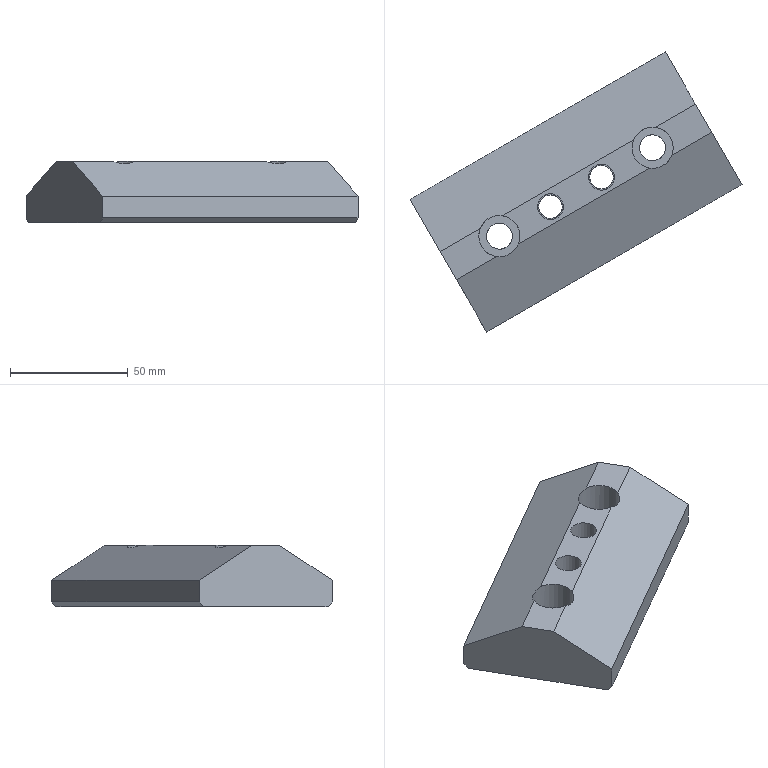Part | NX | features solid 2 | 1 solid | 24 faces | box 140.753 x 118.792 x 26 mm | volume 149536 mm3 | plane 16 | cylinder 8 | commonest cylinder face diameters 11 x4 10 x2 17.5 x2
STEP:
#1=CARTESIAN_POINT('',(-909.878,104.476,-234.));
#2=VERTEX_POINT('',#1);
#3=CARTESIAN_POINT('',(-916.806,116.476,-234.));
#4=VERTEX_POINT('',#3);
#5=CARTESIAN_POINT('',(-917.971,107.804,-234.));
#6=DIRECTION('',(0.,0.,1.));
#7=DIRECTION('',(-0.866,-0.5,0.));
#8=AXIS2_PLACEMENT_3D('',#5,#6,#7);
#9=CIRCLE('',#8,8.75);
#10=EDGE_CURVE('',#2,#4,#9,.T.);
#11=ORIENTED_EDGE('',*,*,#10,.F.);
#12=CARTESIAN_POINT('',(-892.856,114.304,-234.));
#13=VERTEX_POINT('',#12);
#14=CARTESIAN_POINT('',(-892.856,114.304,-234.));
#15=DIRECTION('',(-0.866,-0.5,0.));
#16=VECTOR('',#15,1000.);
#17=LINE('',#14,#16);
#18=EDGE_CURVE('',#13,#2,#17,.T.);
#19=ORIENTED_EDGE('',*,*,#18,.F.);
#20=CARTESIAN_POINT('',(-899.784,126.304,-234.));
#21=VERTEX_POINT('',#20);
#22=CARTESIAN_POINT('',(-899.784,126.304,-234.));
#23=DIRECTION('',(0.5,-0.866,0.));
#24=VECTOR('',#23,1000.);
#25=LINE('',#22,#24);
#26=EDGE_CURVE('',#21,#13,#25,.T.);
#27=ORIENTED_EDGE('',*,*,#26,.F.);
#28=CARTESIAN_POINT('',(-899.784,126.304,-234.));
#29=DIRECTION('',(-0.866,-0.5,0.));
#30=VECTOR('',#29,1000.);
#31=LINE('',#28,#30);
#32=EDGE_CURVE('',#21,#4,#31,.T.);
#33=ORIENTED_EDGE('',*,*,#32,.T.);
#34=EDGE_LOOP('',(#11,#19,#27,#33));
#35=FACE_BOUND('',#34,.T.);
#36=CARTESIAN_POINT('',(-899.784,126.304,-234.));
#37=DIRECTION('',(0.,0.,1.));
#38=DIRECTION('',(-0.5,0.866,0.));
#39=AXIS2_PLACEMENT_3D('',#36,#37,#38);
#40=PLANE('',#39);
#41=ADVANCED_FACE('',(#35),#40,.T.);
#42=CARTESIAN_POINT('',(-944.384,92.554,-234.));
#43=VERTEX_POINT('',#42);
#44=CARTESIAN_POINT('',(-939.621,95.304,-234.));
#45=DIRECTION('',(0.,0.,1.));
#46=DIRECTION('',(-0.866,-0.5,0.));
#47=AXIS2_PLACEMENT_3D('',#44,#45,#46);
#48=CIRCLE('',#47,5.5);
#49=EDGE_CURVE('',#43,#43,#48,.T.);
#50=ORIENTED_EDGE('',*,*,#49,.F.);
#51=EDGE_LOOP('',(#50));
#52=FACE_BOUND('',#51,.T.);
#53=CARTESIAN_POINT('',(-926.063,111.132,-234.));
#54=VERTEX_POINT('',#53);
#55=CARTESIAN_POINT('',(-919.135,99.132,-234.));
#56=VERTEX_POINT('',#55);
#57=CARTESIAN_POINT('',(-917.971,107.804,-234.));
#58=DIRECTION('',(0.,0.,1.));
#59=DIRECTION('',(-0.866,-0.5,0.));
#60=AXIS2_PLACEMENT_3D('',#57,#58,#59);
#61=CIRCLE('',#60,8.75);
#62=EDGE_CURVE('',#54,#56,#61,.T.);
#63=ORIENTED_EDGE('',*,*,#62,.F.);
#64=CARTESIAN_POINT('',(-981.758,78.976,-234.));
#65=VERTEX_POINT('',#64);
#66=CARTESIAN_POINT('',(-899.784,126.304,-234.));
#67=DIRECTION('',(-0.866,-0.5,0.));
#68=VECTOR('',#67,1000.);
#69=LINE('',#66,#68);
#70=EDGE_CURVE('',#54,#65,#69,.T.);
#71=ORIENTED_EDGE('',*,*,#70,.T.);
#72=CARTESIAN_POINT('',(-974.83,66.976,-234.));
#73=VERTEX_POINT('',#72);
#74=CARTESIAN_POINT('',(-982.922,70.304,-234.));
#75=DIRECTION('',(0.,0.,1.));
#76=DIRECTION('',(-0.866,-0.5,0.));
#77=AXIS2_PLACEMENT_3D('',#74,#75,#76);
#78=CIRCLE('',#77,8.75);
#79=EDGE_CURVE('',#73,#65,#78,.T.);
#80=ORIENTED_EDGE('',*,*,#79,.F.);
#81=CARTESIAN_POINT('',(-892.856,114.304,-234.));
#82=DIRECTION('',(-0.866,-0.5,0.));
#83=VECTOR('',#82,1000.);
#84=LINE('',#81,#83);
#85=EDGE_CURVE('',#56,#73,#84,.T.);
#86=ORIENTED_EDGE('',*,*,#85,.F.);
#87=EDGE_LOOP('',(#63,#71,#80,#86));
#88=FACE_BOUND('',#87,.T.);
#89=CARTESIAN_POINT('',(-966.035,80.054,-234.));
#90=VERTEX_POINT('',#89);
#91=CARTESIAN_POINT('',(-961.272,82.804,-234.));
#92=DIRECTION('',(0.,0.,1.));
#93=DIRECTION('',(-0.866,-0.5,0.));
#94=AXIS2_PLACEMENT_3D('',#91,#92,#93);
#95=CIRCLE('',#94,5.5);
#96=EDGE_CURVE('',#90,#90,#95,.T.);
#97=ORIENTED_EDGE('',*,*,#96,.F.);
#98=EDGE_LOOP('',(#97));
#99=FACE_BOUND('',#98,.T.);
#100=CARTESIAN_POINT('',(-899.784,126.304,-234.));
#101=DIRECTION('',(0.,0.,1.));
#102=DIRECTION('',(-0.5,0.866,0.));
#103=AXIS2_PLACEMENT_3D('',#100,#101,#102);
#104=PLANE('',#103);
#105=ADVANCED_FACE('',(#52,#88,#99),#104,.T.);
#106=CARTESIAN_POINT('',(-917.971,107.804,-230.));
#107=DIRECTION('',(-0.25,0.433,-0.866));
#108=DIRECTION('',(0.433,-0.75,-0.5));
#109=AXIS2_PLACEMENT_3D('',#106,#107,#108);
#110=ELLIPSE('',#109,10.104,8.75);
#111=EDGE_CURVE('',#2,#56,#110,.T.);
#112=ORIENTED_EDGE('',*,*,#111,.T.);
#113=ORIENTED_EDGE('',*,*,#85,.T.);
#114=CARTESIAN_POINT('',(-984.087,61.632,-234.));
#115=VERTEX_POINT('',#114);
#116=CARTESIAN_POINT('',(-982.922,70.304,-230.));
#117=DIRECTION('',(-0.25,0.433,-0.866));
#118=DIRECTION('',(0.433,-0.75,-0.5));
#119=AXIS2_PLACEMENT_3D('',#116,#117,#118);
#120=ELLIPSE('',#119,10.104,8.75);
#121=EDGE_CURVE('',#73,#115,#120,.T.);
#122=ORIENTED_EDGE('',*,*,#121,.T.);
#123=CARTESIAN_POINT('',(-1001.109,51.804,-234.));
#124=VERTEX_POINT('',#123);
#125=CARTESIAN_POINT('',(-892.856,114.304,-234.));
#126=DIRECTION('',(-0.866,-0.5,0.));
#127=VECTOR('',#126,1000.);
#128=LINE('',#125,#127);
#129=EDGE_CURVE('',#115,#124,#128,.T.);
#130=ORIENTED_EDGE('',*,*,#129,.T.);
#131=CARTESIAN_POINT('',(-988.323,29.658,-248.764));
#132=VERTEX_POINT('',#131);
#133=CARTESIAN_POINT('',(-1001.109,51.804,-234.));
#134=DIRECTION('',(0.433,-0.75,-0.5));
#135=VECTOR('',#134,1000.);
#136=LINE('',#133,#135);
#137=EDGE_CURVE('',#124,#132,#136,.T.);
#138=ORIENTED_EDGE('',*,*,#137,.T.);
#139=CARTESIAN_POINT('',(-880.07,92.158,-248.764));
#140=VERTEX_POINT('',#139);
#141=CARTESIAN_POINT('',(-880.07,92.158,-248.764));
#142=DIRECTION('',(-0.866,-0.5,0.));
#143=VECTOR('',#142,1000.);
#144=LINE('',#141,#143);
#145=EDGE_CURVE('',#140,#132,#144,.T.);
#146=ORIENTED_EDGE('',*,*,#145,.F.);
#147=CARTESIAN_POINT('',(-892.856,114.304,-234.));
#148=DIRECTION('',(0.433,-0.75,-0.5));
#149=VECTOR('',#148,1000.);
#150=LINE('',#147,#149);
#151=EDGE_CURVE('',#13,#140,#150,.T.);
#152=ORIENTED_EDGE('',*,*,#151,.F.);
#153=ORIENTED_EDGE('',*,*,#18,.T.);
#154=EDGE_LOOP('',(#112,#113,#122,#130,#138,#146,#152,#153));
#155=FACE_BOUND('',#154,.T.);
#156=CARTESIAN_POINT('',(-892.856,114.304,-234.));
#157=DIRECTION('',(0.25,-0.433,0.866));
#158=DIRECTION('',(-0.433,0.75,0.5));
#159=AXIS2_PLACEMENT_3D('',#156,#157,#158);
#160=PLANE('',#159);
#161=ADVANCED_FACE('',(#155),#160,.T.);
#162=CARTESIAN_POINT('',(-880.07,92.158,-258.));
#163=VERTEX_POINT('',#162);
#164=CARTESIAN_POINT('',(-880.07,92.158,-260.));
#165=DIRECTION('',(0.,0.,1.));
#166=VECTOR('',#165,1000.);
#167=LINE('',#164,#166);
#168=EDGE_CURVE('',#163,#140,#167,.T.);
#169=ORIENTED_EDGE('',*,*,#168,.T.);
#170=ORIENTED_EDGE('',*,*,#145,.T.);
#171=CARTESIAN_POINT('',(-988.323,29.658,-258.));
#172=VERTEX_POINT('',#171);
#173=CARTESIAN_POINT('',(-988.323,29.658,-260.));
#174=DIRECTION('',(0.,0.,1.));
#175=VECTOR('',#174,1000.);
#176=LINE('',#173,#175);
#177=EDGE_CURVE('',#172,#132,#176,.T.);
#178=ORIENTED_EDGE('',*,*,#177,.F.);
#179=CARTESIAN_POINT('',(-880.07,92.158,-258.));
#180=DIRECTION('',(-0.866,-0.5,0.));
#181=VECTOR('',#180,1000.);
#182=LINE('',#179,#181);
#183=EDGE_CURVE('',#163,#172,#182,.T.);
#184=ORIENTED_EDGE('',*,*,#183,.F.);
#185=EDGE_LOOP('',(#169,#170,#178,#184));
#186=FACE_BOUND('',#185,.T.);
#187=CARTESIAN_POINT('',(-880.07,92.158,-260.));
#188=DIRECTION('',(-0.5,0.866,0.));
#189=DIRECTION('',(0.,0.,-1.));
#190=AXIS2_PLACEMENT_3D('',#187,#188,#189);
#191=PLANE('',#190);
#192=ADVANCED_FACE('',(#186),#191,.F.);
#193=CARTESIAN_POINT('',(-942.121,99.634,-260.));
#194=VERTEX_POINT('',#193);
#195=CARTESIAN_POINT('',(-939.621,95.304,-260.));
#196=DIRECTION('',(0.,0.,-1.));
#197=DIRECTION('',(-0.5,0.866,0.));
#198=AXIS2_PLACEMENT_3D('',#195,#196,#197);
#199=CIRCLE('',#198,5.);
#200=EDGE_CURVE('',#194,#194,#199,.T.);
#201=ORIENTED_EDGE('',*,*,#200,.F.);
#202=EDGE_LOOP('',(#201));
#203=FACE_BOUND('',#202,.T.);
#204=CARTESIAN_POINT('',(-920.721,112.567,-260.));
#205=VERTEX_POINT('',#204);
#206=CARTESIAN_POINT('',(-917.971,107.804,-260.));
#207=DIRECTION('',(0.,0.,-1.));
#208=DIRECTION('',(-0.5,0.866,0.));
#209=AXIS2_PLACEMENT_3D('',#206,#207,#208);
#210=CIRCLE('',#209,5.5);
#211=EDGE_CURVE('',#205,#205,#210,.T.);
#212=ORIENTED_EDGE('',*,*,#211,.F.);
#213=EDGE_LOOP('',(#212));
#214=FACE_BOUND('',#213,.T.);
#215=CARTESIAN_POINT('',(-963.772,87.134,-260.));
#216=VERTEX_POINT('',#215);
#217=CARTESIAN_POINT('',(-961.272,82.804,-260.));
#218=DIRECTION('',(0.,0.,-1.));
#219=DIRECTION('',(-0.5,0.866,0.));
#220=AXIS2_PLACEMENT_3D('',#217,#218,#219);
#221=CIRCLE('',#220,5.);
#222=EDGE_CURVE('',#216,#216,#221,.T.);
#223=ORIENTED_EDGE('',*,*,#222,.F.);
#224=EDGE_LOOP('',(#223));
#225=FACE_BOUND('',#224,.T.);
#226=CARTESIAN_POINT('',(-985.672,75.067,-260.));
#227=VERTEX_POINT('',#226);
#228=CARTESIAN_POINT('',(-982.922,70.304,-260.));
#229=DIRECTION('',(0.,0.,-1.));
#230=DIRECTION('',(-0.5,0.866,0.));
#231=AXIS2_PLACEMENT_3D('',#228,#229,#230);
#232=CIRCLE('',#231,5.5);
#233=EDGE_CURVE('',#227,#227,#232,.T.);
#234=ORIENTED_EDGE('',*,*,#233,.F.);
#235=EDGE_LOOP('',(#234));
#236=FACE_BOUND('',#235,.T.);
#237=CARTESIAN_POINT('',(-1019.823,84.218,-260.));
#238=VERTEX_POINT('',#237);
#239=CARTESIAN_POINT('',(-989.323,31.391,-260.));
#240=VERTEX_POINT('',#239);
#241=CARTESIAN_POINT('',(-1020.823,85.95,-260.));
#242=DIRECTION('',(0.5,-0.866,0.));
#243=VECTOR('',#242,1000.);
#244=LINE('',#241,#243);
#245=EDGE_CURVE('',#238,#240,#244,.T.);
#246=ORIENTED_EDGE('',*,*,#245,.F.);
#247=CARTESIAN_POINT('',(-911.57,146.718,-260.));
#248=VERTEX_POINT('',#247);
#249=CARTESIAN_POINT('',(-911.57,146.718,-260.));
#250=DIRECTION('',(-0.866,-0.5,0.));
#251=VECTOR('',#250,1000.);
#252=LINE('',#249,#251);
#253=EDGE_CURVE('',#248,#238,#252,.T.);
#254=ORIENTED_EDGE('',*,*,#253,.F.);
#255=CARTESIAN_POINT('',(-881.07,93.891,-260.));
#256=VERTEX_POINT('',#255);
#257=CARTESIAN_POINT('',(-912.57,148.45,-260.));
#258=DIRECTION('',(0.5,-0.866,0.));
#259=VECTOR('',#258,1000.);
#260=LINE('',#257,#259);
#261=EDGE_CURVE('',#248,#256,#260,.T.);
#262=ORIENTED_EDGE('',*,*,#261,.T.);
#263=CARTESIAN_POINT('',(-881.07,93.891,-260.));
#264=DIRECTION('',(0.866,0.5,0.));
#265=VECTOR('',#264,1000.);
#266=LINE('',#263,#265);
#267=EDGE_CURVE('',#240,#256,#266,.T.);
#268=ORIENTED_EDGE('',*,*,#267,.F.);
#269=EDGE_LOOP('',(#246,#254,#262,#268));
#270=FACE_BOUND('',#269,.T.);
#271=CARTESIAN_POINT('',(-912.57,148.45,-260.));
#272=DIRECTION('',(0.,0.,1.));
#273=DIRECTION('',(-0.5,0.866,0.));
#274=AXIS2_PLACEMENT_3D('',#271,#272,#273);
#275=PLANE('',#274);
#276=ADVANCED_FACE('',(#203,#214,#225,#236,#270),#275,.F.);
#277=CARTESIAN_POINT('',(-1020.823,85.95,-248.764));
#278=VERTEX_POINT('',#277);
#279=CARTESIAN_POINT('',(-1020.823,85.95,-258.));
#280=VERTEX_POINT('',#279);
#281=CARTESIAN_POINT('',(-1020.823,85.95,-248.764));
#282=DIRECTION('',(0.,0.,-1.));
#283=VECTOR('',#282,1000.);
#284=LINE('',#281,#283);
#285=EDGE_CURVE('',#278,#280,#284,.T.);
#286=ORIENTED_EDGE('',*,*,#285,.F.);
#287=CARTESIAN_POINT('',(-912.57,148.45,-248.764));
#288=VERTEX_POINT('',#287);
#289=CARTESIAN_POINT('',(-912.57,148.45,-248.764));
#290=DIRECTION('',(-0.866,-0.5,0.));
#291=VECTOR('',#290,1000.);
#292=LINE('',#289,#291);
#293=EDGE_CURVE('',#288,#278,#292,.T.);
#294=ORIENTED_EDGE('',*,*,#293,.F.);
#295=CARTESIAN_POINT('',(-912.57,148.45,-258.));
#296=VERTEX_POINT('',#295);
#297=CARTESIAN_POINT('',(-912.57,148.45,-248.764));
#298=DIRECTION('',(0.,0.,-1.));
#299=VECTOR('',#298,1000.);
#300=LINE('',#297,#299);
#301=EDGE_CURVE('',#288,#296,#300,.T.);
#302=ORIENTED_EDGE('',*,*,#301,.T.);
#303=CARTESIAN_POINT('',(-912.57,148.45,-258.));
#304=DIRECTION('',(0.866,0.5,0.));
#305=VECTOR('',#304,1000.);
#306=LINE('',#303,#305);
#307=EDGE_CURVE('',#280,#296,#306,.T.);
#308=ORIENTED_EDGE('',*,*,#307,.F.);
#309=EDGE_LOOP('',(#286,#294,#302,#308));
#310=FACE_BOUND('',#309,.T.);
#311=CARTESIAN_POINT('',(-912.57,148.45,-248.764));
#312=DIRECTION('',(0.5,-0.866,0.));
#313=DIRECTION('',(0.,0.,1.));
#314=AXIS2_PLACEMENT_3D('',#311,#312,#313);
#315=PLANE('',#314);
#316=ADVANCED_FACE('',(#310),#315,.F.);
#317=CARTESIAN_POINT('',(-917.971,107.804,-230.));
#318=DIRECTION('',(0.25,-0.433,-0.866));
#319=DIRECTION('',(-0.433,0.75,-0.5));
#320=AXIS2_PLACEMENT_3D('',#317,#318,#319);
#321=ELLIPSE('',#320,10.104,8.75);
#322=EDGE_CURVE('',#54,#4,#321,.T.);
#323=ORIENTED_EDGE('',*,*,#322,.T.);
#324=ORIENTED_EDGE('',*,*,#32,.F.);
#325=CARTESIAN_POINT('',(-912.57,148.45,-248.764));
#326=DIRECTION('',(0.433,-0.75,0.5));
#327=VECTOR('',#326,1000.);
#328=LINE('',#325,#327);
#329=EDGE_CURVE('',#288,#21,#328,.T.);
#330=ORIENTED_EDGE('',*,*,#329,.F.);
#331=ORIENTED_EDGE('',*,*,#293,.T.);
#332=CARTESIAN_POINT('',(-1008.037,63.804,-234.));
#333=VERTEX_POINT('',#332);
#334=CARTESIAN_POINT('',(-1020.823,85.95,-248.764));
#335=DIRECTION('',(0.433,-0.75,0.5));
#336=VECTOR('',#335,1000.);
#337=LINE('',#334,#336);
#338=EDGE_CURVE('',#278,#333,#337,.T.);
#339=ORIENTED_EDGE('',*,*,#338,.T.);
#340=CARTESIAN_POINT('',(-991.015,73.632,-234.));
#341=VERTEX_POINT('',#340);
#342=CARTESIAN_POINT('',(-899.784,126.304,-234.));
#343=DIRECTION('',(-0.866,-0.5,0.));
#344=VECTOR('',#343,1000.);
#345=LINE('',#342,#344);
#346=EDGE_CURVE('',#341,#333,#345,.T.);
#347=ORIENTED_EDGE('',*,*,#346,.F.);
#348=CARTESIAN_POINT('',(-982.922,70.304,-230.));
#349=DIRECTION('',(0.25,-0.433,-0.866));
#350=DIRECTION('',(-0.433,0.75,-0.5));
#351=AXIS2_PLACEMENT_3D('',#348,#349,#350);
#352=ELLIPSE('',#351,10.104,8.75);
#353=EDGE_CURVE('',#341,#65,#352,.T.);
#354=ORIENTED_EDGE('',*,*,#353,.T.);
#355=ORIENTED_EDGE('',*,*,#70,.F.);
#356=EDGE_LOOP('',(#323,#324,#330,#331,#339,#347,#354,#355));
#357=FACE_BOUND('',#356,.T.);
#358=CARTESIAN_POINT('',(-912.57,148.45,-248.764));
#359=DIRECTION('',(-0.25,0.433,0.866));
#360=DIRECTION('',(-0.433,0.75,-0.5));
#361=AXIS2_PLACEMENT_3D('',#358,#359,#360);
#362=PLANE('',#361);
#363=ADVANCED_FACE('',(#357),#362,.T.);
#364=CARTESIAN_POINT('',(-982.922,70.304,-234.));
#365=DIRECTION('',(0.,0.,-1.));
#366=DIRECTION('',(-0.5,0.866,0.));
#367=AXIS2_PLACEMENT_3D('',#364,#365,#366);
#368=CIRCLE('',#367,8.75);
#369=EDGE_CURVE('',#115,#341,#368,.T.);
#370=ORIENTED_EDGE('',*,*,#369,.T.);
#371=ORIENTED_EDGE('',*,*,#346,.T.);
#372=CARTESIAN_POINT('',(-1008.037,63.804,-234.));
#373=DIRECTION('',(0.5,-0.866,0.));
#374=VECTOR('',#373,1000.);
#375=LINE('',#372,#374);
#376=EDGE_CURVE('',#333,#124,#375,.T.);
#377=ORIENTED_EDGE('',*,*,#376,.T.);
#378=ORIENTED_EDGE('',*,*,#129,.F.);
#379=EDGE_LOOP('',(#370,#371,#377,#378));
#380=FACE_BOUND('',#379,.T.);
#381=CARTESIAN_POINT('',(-899.784,126.304,-234.));
#382=DIRECTION('',(0.,0.,1.));
#383=DIRECTION('',(-0.5,0.866,0.));
#384=AXIS2_PLACEMENT_3D('',#381,#382,#383);
#385=PLANE('',#384);
#386=ADVANCED_FACE('',(#380),#385,.T.);
#387=ORIENTED_EDGE('',*,*,#261,.F.);
#388=CARTESIAN_POINT('',(-911.445,146.502,-260.25));
#389=DIRECTION('',(-0.3536,0.6124,0.7071));
#390=VECTOR('',#389,1000.);
#391=LINE('',#388,#390);
#392=EDGE_CURVE('',#296,#248,#391,.F.);
#393=ORIENTED_EDGE('',*,*,#392,.F.);
#394=ORIENTED_EDGE('',*,*,#301,.F.);
#395=ORIENTED_EDGE('',*,*,#329,.T.);
#396=ORIENTED_EDGE('',*,*,#26,.T.);
#397=ORIENTED_EDGE('',*,*,#151,.T.);
#398=ORIENTED_EDGE('',*,*,#168,.F.);
#399=CARTESIAN_POINT('',(-881.195,94.107,-260.25));
#400=DIRECTION('',(-0.3536,0.6124,-0.7071));
#401=VECTOR('',#400,1000.);
#402=LINE('',#399,#401);
#403=EDGE_CURVE('',#256,#163,#402,.F.);
#404=ORIENTED_EDGE('',*,*,#403,.F.);
#405=EDGE_LOOP('',(#387,#393,#394,#395,#396,#397,#398,#404));
#406=FACE_BOUND('',#405,.T.);
#407=CARTESIAN_POINT('',(-896.32,120.304,-230.));
#408=DIRECTION('',(0.866,0.5,0.));
#409=DIRECTION('',(0.,0.,-1.));
#410=AXIS2_PLACEMENT_3D('',#407,#408,#409);
#411=PLANE('',#410);
#412=ADVANCED_FACE('',(#406),#411,.T.);
#413=ORIENTED_EDGE('',*,*,#177,.T.);
#414=ORIENTED_EDGE('',*,*,#137,.F.);
#415=ORIENTED_EDGE('',*,*,#376,.F.);
#416=ORIENTED_EDGE('',*,*,#338,.F.);
#417=ORIENTED_EDGE('',*,*,#285,.T.);
#418=CARTESIAN_POINT('',(-1019.823,84.218,-260.));
#419=DIRECTION('',(0.3536,-0.6124,-0.7071));
#420=VECTOR('',#419,1000.);
#421=LINE('',#418,#420);
#422=EDGE_CURVE('',#238,#280,#421,.F.);
#423=ORIENTED_EDGE('',*,*,#422,.F.);
#424=ORIENTED_EDGE('',*,*,#245,.T.);
#425=CARTESIAN_POINT('',(-988.323,29.658,-258.));
#426=DIRECTION('',(0.3536,-0.6124,0.7071));
#427=VECTOR('',#426,1000.);
#428=LINE('',#425,#427);
#429=EDGE_CURVE('',#172,#240,#428,.F.);
#430=ORIENTED_EDGE('',*,*,#429,.F.);
#431=EDGE_LOOP('',(#413,#414,#415,#416,#417,#423,#424,#430));
#432=FACE_BOUND('',#431,.T.);
#433=CARTESIAN_POINT('',(-1004.573,57.804,-230.));
#434=DIRECTION('',(0.866,0.5,0.));
#435=DIRECTION('',(0.,0.,-1.));
#436=AXIS2_PLACEMENT_3D('',#433,#434,#435);
#437=PLANE('',#436);
#438=ADVANCED_FACE('',(#432),#437,.F.);
#439=CARTESIAN_POINT('',(-987.686,67.554,-250.));
#440=VERTEX_POINT('',#439);
#441=CARTESIAN_POINT('',(-982.922,70.304,-250.));
#442=DIRECTION('',(0.,0.,1.));
#443=DIRECTION('',(-0.866,-0.5,0.));
#444=AXIS2_PLACEMENT_3D('',#441,#442,#443);
#445=CIRCLE('',#444,5.5);
#446=EDGE_CURVE('',#440,#440,#445,.T.);
#447=ORIENTED_EDGE('',*,*,#446,.T.);
#448=EDGE_LOOP('',(#447));
#449=FACE_BOUND('',#448,.T.);
#450=ORIENTED_EDGE('',*,*,#233,.T.);
#451=EDGE_LOOP('',(#450));
#452=FACE_BOUND('',#451,.T.);
#453=CARTESIAN_POINT('',(-982.922,70.304,-264.));
#454=DIRECTION('',(0.,0.,-1.));
#455=DIRECTION('',(-0.866,-0.5,0.));
#456=AXIS2_PLACEMENT_3D('',#453,#454,#455);
#457=CYLINDRICAL_SURFACE('',#456,5.5);
#458=ADVANCED_FACE('',(#449,#452),#457,.F.);
#459=ORIENTED_EDGE('',*,*,#446,.F.);
#460=EDGE_LOOP('',(#459));
#461=FACE_BOUND('',#460,.T.);
#462=CARTESIAN_POINT('',(-990.5,65.929,-250.));
#463=VERTEX_POINT('',#462);
#464=CARTESIAN_POINT('',(-982.922,70.304,-250.));
#465=DIRECTION('',(0.,0.,1.));
#466=DIRECTION('',(-0.866,-0.5,0.));
#467=AXIS2_PLACEMENT_3D('',#464,#465,#466);
#468=CIRCLE('',#467,8.75);
#469=EDGE_CURVE('',#463,#463,#468,.T.);
#470=ORIENTED_EDGE('',*,*,#469,.T.);
#471=EDGE_LOOP('',(#470));
#472=FACE_BOUND('',#471,.T.);
#473=CARTESIAN_POINT('',(-982.922,70.304,-250.));
#474=DIRECTION('',(0.,0.,-1.));
#475=DIRECTION('',(-0.866,-0.5,0.));
#476=AXIS2_PLACEMENT_3D('',#473,#474,#475);
#477=PLANE('',#476);
#478=ADVANCED_FACE('',(#461,#472),#477,.F.);
#479=ORIENTED_EDGE('',*,*,#121,.F.);
#480=ORIENTED_EDGE('',*,*,#79,.T.);
#481=ORIENTED_EDGE('',*,*,#353,.F.);
#482=ORIENTED_EDGE('',*,*,#369,.F.);
#483=EDGE_LOOP('',(#479,#480,#481,#482));
#484=FACE_BOUND('',#483,.T.);
#485=ORIENTED_EDGE('',*,*,#469,.F.);
#486=EDGE_LOOP('',(#485));
#487=FACE_BOUND('',#486,.T.);
#488=CARTESIAN_POINT('',(-982.922,70.304,-234.));
#489=DIRECTION('',(0.,0.,-1.));
#490=DIRECTION('',(-0.866,-0.5,0.));
#491=AXIS2_PLACEMENT_3D('',#488,#489,#490);
#492=CYLINDRICAL_SURFACE('',#491,8.75);
#493=ADVANCED_FACE('',(#484,#487),#492,.F.);
#494=CARTESIAN_POINT('',(-965.602,80.304,-245.));
#495=VERTEX_POINT('',#494);
#496=CARTESIAN_POINT('',(-961.272,82.804,-245.));
#497=DIRECTION('',(0.,0.,1.));
#498=DIRECTION('',(-0.866,-0.5,0.));
#499=AXIS2_PLACEMENT_3D('',#496,#497,#498);
#500=CIRCLE('',#499,5.);
#501=EDGE_CURVE('',#495,#495,#500,.T.);
#502=ORIENTED_EDGE('',*,*,#501,.T.);
#503=EDGE_LOOP('',(#502));
#504=FACE_BOUND('',#503,.T.);
#505=ORIENTED_EDGE('',*,*,#222,.T.);
#506=EDGE_LOOP('',(#505));
#507=FACE_BOUND('',#506,.T.);
#508=CARTESIAN_POINT('',(-961.272,82.804,-264.));
#509=DIRECTION('',(0.,0.,-1.));
#510=DIRECTION('',(-0.866,-0.5,0.));
#511=AXIS2_PLACEMENT_3D('',#508,#509,#510);
#512=CYLINDRICAL_SURFACE('',#511,5.);
#513=ADVANCED_FACE('',(#504,#507),#512,.F.);
#514=ORIENTED_EDGE('',*,*,#501,.F.);
#515=EDGE_LOOP('',(#514));
#516=FACE_BOUND('',#515,.T.);
#517=CARTESIAN_POINT('',(-966.035,80.054,-245.));
#518=VERTEX_POINT('',#517);
#519=CARTESIAN_POINT('',(-961.272,82.804,-245.));
#520=DIRECTION('',(0.,0.,1.));
#521=DIRECTION('',(-0.866,-0.5,0.));
#522=AXIS2_PLACEMENT_3D('',#519,#520,#521);
#523=CIRCLE('',#522,5.5);
#524=EDGE_CURVE('',#518,#518,#523,.T.);
#525=ORIENTED_EDGE('',*,*,#524,.T.);
#526=EDGE_LOOP('',(#525));
#527=FACE_BOUND('',#526,.T.);
#528=CARTESIAN_POINT('',(-961.272,82.804,-245.));
#529=DIRECTION('',(0.,0.,-1.));
#530=DIRECTION('',(-0.866,-0.5,0.));
#531=AXIS2_PLACEMENT_3D('',#528,#529,#530);
#532=PLANE('',#531);
#533=ADVANCED_FACE('',(#516,#527),#532,.F.);
#534=ORIENTED_EDGE('',*,*,#524,.F.);
#535=EDGE_LOOP('',(#534));
#536=FACE_BOUND('',#535,.T.);
#537=ORIENTED_EDGE('',*,*,#96,.T.);
#538=EDGE_LOOP('',(#537));
#539=FACE_BOUND('',#538,.T.);
#540=CARTESIAN_POINT('',(-961.272,82.804,-234.));
#541=DIRECTION('',(0.,0.,-1.));
#542=DIRECTION('',(-0.866,-0.5,0.));
#543=AXIS2_PLACEMENT_3D('',#540,#541,#542);
#544=CYLINDRICAL_SURFACE('',#543,5.5);
#545=ADVANCED_FACE('',(#536,#539),#544,.F.);
#546=CARTESIAN_POINT('',(-922.734,105.054,-250.));
#547=VERTEX_POINT('',#546);
#548=CARTESIAN_POINT('',(-917.971,107.804,-250.));
#549=DIRECTION('',(0.,0.,1.));
#550=DIRECTION('',(-0.866,-0.5,0.));
#551=AXIS2_PLACEMENT_3D('',#548,#549,#550);
#552=CIRCLE('',#551,5.5);
#553=EDGE_CURVE('',#547,#547,#552,.T.);
#554=ORIENTED_EDGE('',*,*,#553,.T.);
#555=EDGE_LOOP('',(#554));
#556=FACE_BOUND('',#555,.T.);
#557=ORIENTED_EDGE('',*,*,#211,.T.);
#558=EDGE_LOOP('',(#557));
#559=FACE_BOUND('',#558,.T.);
#560=CARTESIAN_POINT('',(-917.971,107.804,-264.));
#561=DIRECTION('',(0.,0.,-1.));
#562=DIRECTION('',(-0.866,-0.5,0.));
#563=AXIS2_PLACEMENT_3D('',#560,#561,#562);
#564=CYLINDRICAL_SURFACE('',#563,5.5);
#565=ADVANCED_FACE('',(#556,#559),#564,.F.);
#566=ORIENTED_EDGE('',*,*,#553,.F.);
#567=EDGE_LOOP('',(#566));
#568=FACE_BOUND('',#567,.T.);
#569=CARTESIAN_POINT('',(-925.548,103.429,-250.));
#570=VERTEX_POINT('',#569);
#571=CARTESIAN_POINT('',(-917.971,107.804,-250.));
#572=DIRECTION('',(0.,0.,1.));
#573=DIRECTION('',(-0.866,-0.5,0.));
#574=AXIS2_PLACEMENT_3D('',#571,#572,#573);
#575=CIRCLE('',#574,8.75);
#576=EDGE_CURVE('',#570,#570,#575,.T.);
#577=ORIENTED_EDGE('',*,*,#576,.T.);
#578=EDGE_LOOP('',(#577));
#579=FACE_BOUND('',#578,.T.);
#580=CARTESIAN_POINT('',(-917.971,107.804,-250.));
#581=DIRECTION('',(0.,0.,-1.));
#582=DIRECTION('',(-0.866,-0.5,0.));
#583=AXIS2_PLACEMENT_3D('',#580,#581,#582);
#584=PLANE('',#583);
#585=ADVANCED_FACE('',(#568,#579),#584,.F.);
#586=ORIENTED_EDGE('',*,*,#111,.F.);
#587=ORIENTED_EDGE('',*,*,#10,.T.);
#588=ORIENTED_EDGE('',*,*,#322,.F.);
#589=ORIENTED_EDGE('',*,*,#62,.T.);
#590=EDGE_LOOP('',(#586,#587,#588,#589));
#591=FACE_BOUND('',#590,.T.);
#592=ORIENTED_EDGE('',*,*,#576,.F.);
#593=EDGE_LOOP('',(#592));
#594=FACE_BOUND('',#593,.T.);
#595=CARTESIAN_POINT('',(-917.971,107.804,-234.));
#596=DIRECTION('',(0.,0.,-1.));
#597=DIRECTION('',(-0.866,-0.5,0.));
#598=AXIS2_PLACEMENT_3D('',#595,#596,#597);
#599=CYLINDRICAL_SURFACE('',#598,8.75);
#600=ADVANCED_FACE('',(#591,#594),#599,.F.);
#601=CARTESIAN_POINT('',(-943.951,92.804,-245.));
#602=VERTEX_POINT('',#601);
#603=CARTESIAN_POINT('',(-939.621,95.304,-245.));
#604=DIRECTION('',(0.,0.,1.));
#605=DIRECTION('',(-0.866,-0.5,0.));
#606=AXIS2_PLACEMENT_3D('',#603,#604,#605);
#607=CIRCLE('',#606,5.);
#608=EDGE_CURVE('',#602,#602,#607,.T.);
#609=ORIENTED_EDGE('',*,*,#608,.T.);
#610=EDGE_LOOP('',(#609));
#611=FACE_BOUND('',#610,.T.);
#612=ORIENTED_EDGE('',*,*,#200,.T.);
#613=EDGE_LOOP('',(#612));
#614=FACE_BOUND('',#613,.T.);
#615=CARTESIAN_POINT('',(-939.621,95.304,-264.));
#616=DIRECTION('',(0.,0.,-1.));
#617=DIRECTION('',(-0.866,-0.5,0.));
#618=AXIS2_PLACEMENT_3D('',#615,#616,#617);
#619=CYLINDRICAL_SURFACE('',#618,5.);
#620=ADVANCED_FACE('',(#611,#614),#619,.F.);
#621=ORIENTED_EDGE('',*,*,#608,.F.);
#622=EDGE_LOOP('',(#621));
#623=FACE_BOUND('',#622,.T.);
#624=CARTESIAN_POINT('',(-944.384,92.554,-245.));
#625=VERTEX_POINT('',#624);
#626=CARTESIAN_POINT('',(-939.621,95.304,-245.));
#627=DIRECTION('',(0.,0.,1.));
#628=DIRECTION('',(-0.866,-0.5,0.));
#629=AXIS2_PLACEMENT_3D('',#626,#627,#628);
#630=CIRCLE('',#629,5.5);
#631=EDGE_CURVE('',#625,#625,#630,.T.);
#632=ORIENTED_EDGE('',*,*,#631,.T.);
#633=EDGE_LOOP('',(#632));
#634=FACE_BOUND('',#633,.T.);
#635=CARTESIAN_POINT('',(-939.621,95.304,-245.));
#636=DIRECTION('',(0.,0.,-1.));
#637=DIRECTION('',(-0.866,-0.5,0.));
#638=AXIS2_PLACEMENT_3D('',#635,#636,#637);
#639=PLANE('',#638);
#640=ADVANCED_FACE('',(#623,#634),#639,.F.);
#641=ORIENTED_EDGE('',*,*,#631,.F.);
#642=EDGE_LOOP('',(#641));
#643=FACE_BOUND('',#642,.T.);
#644=ORIENTED_EDGE('',*,*,#49,.T.);
#645=EDGE_LOOP('',(#644));
#646=FACE_BOUND('',#645,.T.);
#647=CARTESIAN_POINT('',(-939.621,95.304,-234.));
#648=DIRECTION('',(0.,0.,-1.));
#649=DIRECTION('',(-0.866,-0.5,0.));
#650=AXIS2_PLACEMENT_3D('',#647,#648,#649);
#651=CYLINDRICAL_SURFACE('',#650,5.5);
#652=ADVANCED_FACE('',(#643,#646),#651,.F.);
#653=ORIENTED_EDGE('',*,*,#403,.T.);
#654=ORIENTED_EDGE('',*,*,#183,.T.);
#655=ORIENTED_EDGE('',*,*,#429,.T.);
#656=ORIENTED_EDGE('',*,*,#267,.T.);
#657=EDGE_LOOP('',(#653,#654,#655,#656));
#658=FACE_BOUND('',#657,.T.);
#659=CARTESIAN_POINT('',(-880.07,92.158,-258.));
#660=DIRECTION('',(-0.3536,0.6124,0.7071));
#661=DIRECTION('',(-0.3536,0.6124,-0.7071));
#662=AXIS2_PLACEMENT_3D('',#659,#660,#661);
#663=PLANE('',#662);
#664=ADVANCED_FACE('',(#658),#663,.F.);
#665=ORIENTED_EDGE('',*,*,#392,.T.);
#666=ORIENTED_EDGE('',*,*,#253,.T.);
#667=ORIENTED_EDGE('',*,*,#422,.T.);
#668=ORIENTED_EDGE('',*,*,#307,.T.);
#669=EDGE_LOOP('',(#665,#666,#667,#668));
#670=FACE_BOUND('',#669,.T.);
#671=CARTESIAN_POINT('',(-911.57,146.718,-260.));
#672=DIRECTION('',(0.3536,-0.6124,0.7071));
#673=DIRECTION('',(-0.3536,0.6124,0.7071));
#674=AXIS2_PLACEMENT_3D('',#671,#672,#673);
#675=PLANE('',#674);
#676=ADVANCED_FACE('',(#670),#675,.F.);
#677=CLOSED_SHELL('',(#41,#105,#161,#192,#276,#316,#363,#386,#412,#438,#458,#478,#493,#513,#533,#545,#565,#585,#600,#620,#640,#652,#664,#676));
#678=MANIFOLD_SOLID_BREP('',#677);
#679=(LENGTH_UNIT()NAMED_UNIT(*)SI_UNIT(.MILLI.,.METRE.));
#680=UNCERTAINTY_MEASURE_WITH_UNIT(LENGTH_MEASURE(0.00001),#679,'','');
#681=(NAMED_UNIT(*)PLANE_ANGLE_UNIT()SI_UNIT($,.RADIAN.));
#682=(NAMED_UNIT(*)SI_UNIT($,.STERADIAN.)SOLID_ANGLE_UNIT());
#683=(GEOMETRIC_REPRESENTATION_CONTEXT(3)GLOBAL_UNCERTAINTY_ASSIGNED_CONTEXT((#680))GLOBAL_UNIT_ASSIGNED_CONTEXT((#679,#681,#682))REPRESENTATION_CONTEXT('',''));
#684=ADVANCED_BREP_SHAPE_REPRESENTATION('',(#678),#683);